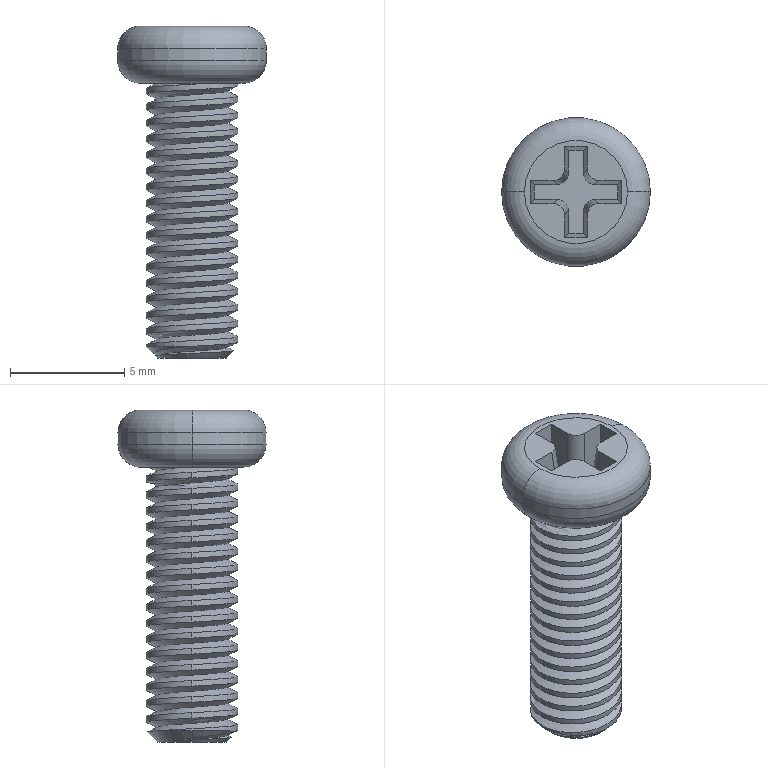Part | SolidWorks | features Fillet 2, ICE 2, Chamfer 1, Extrusion 1, Helix 1, SweepCut 1 | 1 solid | 66 faces | box 6.5 x 6.5 x 14.5 mm | volume 192.159 mm3 | cylinder 41 | plane 16 | torus 4 | cone 3 | spline 2 | commonest cylinder face diameters 4 x35 1 x4 6.5 x2